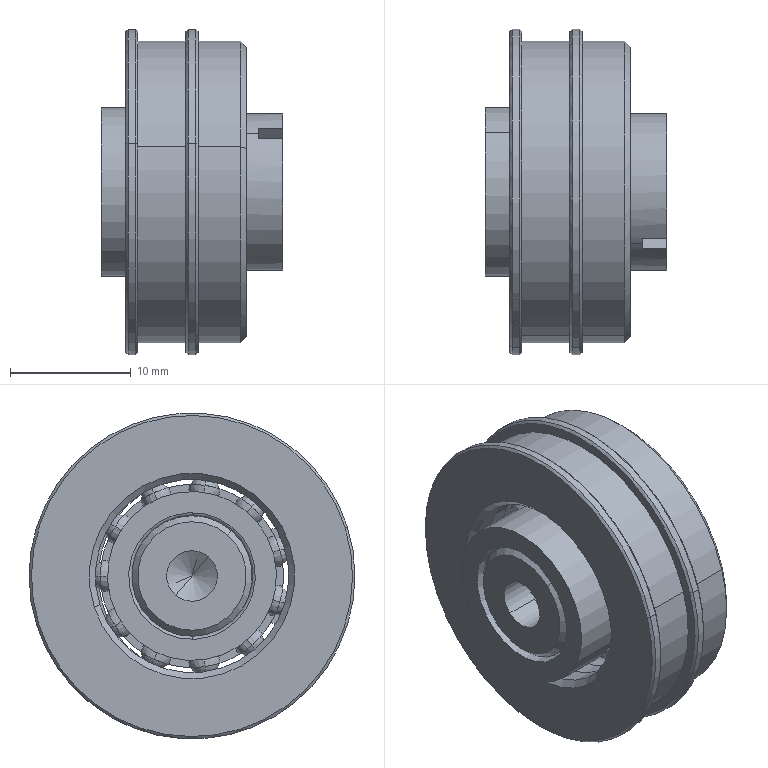Part | SolidWorks | 5 solids | 254 faces | box 15 x 27 x 27 mm | volume 4689 mm3 | sphere 88 | cylinder 57 | plane 47 | torus 44 | cone 18 | commonest cylinder face diameters 19 x6 2 x4 10 x4 12.6 x4 16.4 x4 25 x4